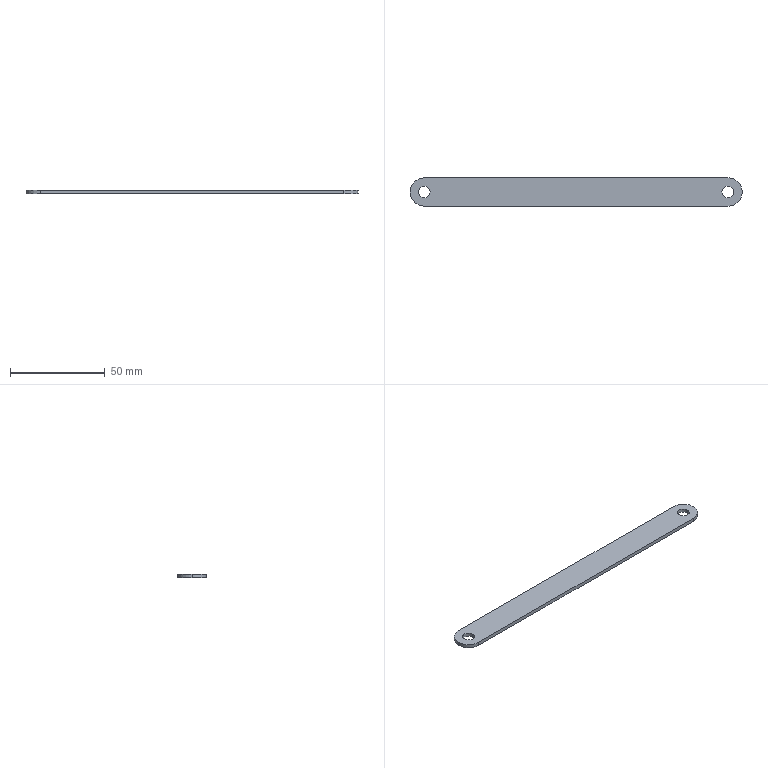Part | SolidWorks | features FlatPattern 1, SMBaseFlange 1, SheetMetal 1 | 1 solid | 11 faces | box 175 x 15 x 2 mm | volume 5033 mm3 | cylinder 7 | plane 4 | commonest cylinder face diameters 6.2 x4 15 x3
STEP:
#1=CARTESIAN_POINT('',(-3.1,7.5,2.));
#2=VERTEX_POINT('',#1);
#3=CARTESIAN_POINT('',(3.1,7.5,2.));
#4=VERTEX_POINT('',#3);
#5=CARTESIAN_POINT('',(0.,7.5,2.));
#6=DIRECTION('',(0.,0.,1.));
#7=DIRECTION('',(1.,0.,0.));
#8=AXIS2_PLACEMENT_3D('',#5,#6,#7);
#9=CIRCLE('',#8,3.1);
#10=EDGE_CURVE('',#2,#4,#9,.T.);
#11=ORIENTED_EDGE('',*,*,#10,.T.);
#12=CARTESIAN_POINT('',(3.1,7.5,0.));
#13=VERTEX_POINT('',#12);
#14=CARTESIAN_POINT('',(3.1,7.5,2.));
#15=DIRECTION('',(0.,0.,-1.));
#16=VECTOR('',#15,1000.);
#17=LINE('',#14,#16);
#18=EDGE_CURVE('',#4,#13,#17,.T.);
#19=ORIENTED_EDGE('',*,*,#18,.T.);
#20=CARTESIAN_POINT('',(-3.1,7.5,0.));
#21=VERTEX_POINT('',#20);
#22=CARTESIAN_POINT('',(0.,7.5,0.));
#23=DIRECTION('',(0.,0.,1.));
#24=DIRECTION('',(1.,0.,0.));
#25=AXIS2_PLACEMENT_3D('',#22,#23,#24);
#26=CIRCLE('',#25,3.1);
#27=EDGE_CURVE('',#21,#13,#26,.T.);
#28=ORIENTED_EDGE('',*,*,#27,.F.);
#29=CARTESIAN_POINT('',(-3.1,7.5,2.));
#30=DIRECTION('',(0.,0.,-1.));
#31=VECTOR('',#30,1000.);
#32=LINE('',#29,#31);
#33=EDGE_CURVE('',#2,#21,#32,.T.);
#34=ORIENTED_EDGE('',*,*,#33,.F.);
#35=EDGE_LOOP('',(#11,#19,#28,#34));
#36=FACE_OUTER_BOUND('',#35,.T.);
#37=CARTESIAN_POINT('',(0.,7.5,2.));
#38=DIRECTION('',(0.,0.,-1.));
#39=DIRECTION('',(-1.,0.,0.));
#40=AXIS2_PLACEMENT_3D('',#37,#38,#39);
#41=CYLINDRICAL_SURFACE('',#40,3.1);
#42=ADVANCED_FACE('',(#36),#41,.F.);
#43=CARTESIAN_POINT('',(-163.1,7.5,2.));
#44=VERTEX_POINT('',#43);
#45=CARTESIAN_POINT('',(-156.9,7.5,2.));
#46=VERTEX_POINT('',#45);
#47=CARTESIAN_POINT('',(-160.,7.5,2.));
#48=DIRECTION('',(0.,0.,1.));
#49=DIRECTION('',(1.,0.,0.));
#50=AXIS2_PLACEMENT_3D('',#47,#48,#49);
#51=CIRCLE('',#50,3.1);
#52=EDGE_CURVE('',#44,#46,#51,.T.);
#53=ORIENTED_EDGE('',*,*,#52,.T.);
#54=CARTESIAN_POINT('',(-156.9,7.5,0.));
#55=VERTEX_POINT('',#54);
#56=CARTESIAN_POINT('',(-156.9,7.5,2.));
#57=DIRECTION('',(0.,0.,-1.));
#58=VECTOR('',#57,1000.);
#59=LINE('',#56,#58);
#60=EDGE_CURVE('',#46,#55,#59,.T.);
#61=ORIENTED_EDGE('',*,*,#60,.T.);
#62=CARTESIAN_POINT('',(-163.1,7.5,0.));
#63=VERTEX_POINT('',#62);
#64=CARTESIAN_POINT('',(-160.,7.5,0.));
#65=DIRECTION('',(0.,0.,1.));
#66=DIRECTION('',(1.,0.,0.));
#67=AXIS2_PLACEMENT_3D('',#64,#65,#66);
#68=CIRCLE('',#67,3.1);
#69=EDGE_CURVE('',#63,#55,#68,.T.);
#70=ORIENTED_EDGE('',*,*,#69,.F.);
#71=CARTESIAN_POINT('',(-163.1,7.5,2.));
#72=DIRECTION('',(0.,0.,-1.));
#73=VECTOR('',#72,1000.);
#74=LINE('',#71,#73);
#75=EDGE_CURVE('',#44,#63,#74,.T.);
#76=ORIENTED_EDGE('',*,*,#75,.F.);
#77=EDGE_LOOP('',(#53,#61,#70,#76));
#78=FACE_OUTER_BOUND('',#77,.T.);
#79=CARTESIAN_POINT('',(-160.,7.5,2.));
#80=DIRECTION('',(0.,0.,-1.));
#81=DIRECTION('',(-1.,0.,0.));
#82=AXIS2_PLACEMENT_3D('',#79,#80,#81);
#83=CYLINDRICAL_SURFACE('',#82,3.1);
#84=ADVANCED_FACE('',(#78),#83,.F.);
#85=CARTESIAN_POINT('',(-167.5,7.5,2.));
#86=VERTEX_POINT('',#85);
#87=CARTESIAN_POINT('',(-160.,0.,2.));
#88=VERTEX_POINT('',#87);
#89=CARTESIAN_POINT('',(-160.,7.5,2.));
#90=DIRECTION('',(0.,0.,1.));
#91=DIRECTION('',(1.,0.,0.));
#92=AXIS2_PLACEMENT_3D('',#89,#90,#91);
#93=CIRCLE('',#92,7.5);
#94=EDGE_CURVE('',#86,#88,#93,.T.);
#95=ORIENTED_EDGE('',*,*,#94,.F.);
#96=CARTESIAN_POINT('',(-167.5,7.5,0.));
#97=VERTEX_POINT('',#96);
#98=CARTESIAN_POINT('',(-167.5,7.5,2.));
#99=DIRECTION('',(0.,0.,-1.));
#100=VECTOR('',#99,1000.);
#101=LINE('',#98,#100);
#102=EDGE_CURVE('',#86,#97,#101,.T.);
#103=ORIENTED_EDGE('',*,*,#102,.T.);
#104=CARTESIAN_POINT('',(-160.,0.,0.));
#105=VERTEX_POINT('',#104);
#106=CARTESIAN_POINT('',(-160.,7.5,0.));
#107=DIRECTION('',(0.,0.,1.));
#108=DIRECTION('',(1.,0.,0.));
#109=AXIS2_PLACEMENT_3D('',#106,#107,#108);
#110=CIRCLE('',#109,7.5);
#111=EDGE_CURVE('',#97,#105,#110,.T.);
#112=ORIENTED_EDGE('',*,*,#111,.T.);
#113=CARTESIAN_POINT('',(-160.,0.,2.));
#114=DIRECTION('',(0.,0.,-1.));
#115=VECTOR('',#114,1000.);
#116=LINE('',#113,#115);
#117=EDGE_CURVE('',#88,#105,#116,.T.);
#118=ORIENTED_EDGE('',*,*,#117,.F.);
#119=EDGE_LOOP('',(#95,#103,#112,#118));
#120=FACE_OUTER_BOUND('',#119,.T.);
#121=CARTESIAN_POINT('',(-160.,7.5,2.));
#122=DIRECTION('',(0.,0.,-1.));
#123=DIRECTION('',(-1.,0.,0.));
#124=AXIS2_PLACEMENT_3D('',#121,#122,#123);
#125=CYLINDRICAL_SURFACE('',#124,7.5);
#126=ADVANCED_FACE('',(#120),#125,.T.);
#127=ORIENTED_EDGE('',*,*,#52,.F.);
#128=CARTESIAN_POINT('',(-160.,7.5,2.));
#129=DIRECTION('',(0.,0.,1.));
#130=DIRECTION('',(1.,0.,0.));
#131=AXIS2_PLACEMENT_3D('',#128,#129,#130);
#132=CIRCLE('',#131,3.1);
#133=EDGE_CURVE('',#46,#44,#132,.T.);
#134=ORIENTED_EDGE('',*,*,#133,.F.);
#135=EDGE_LOOP('',(#127,#134));
#136=FACE_BOUND('',#135,.T.);
#137=CARTESIAN_POINT('',(0.,0.,2.));
#138=VERTEX_POINT('',#137);
#139=CARTESIAN_POINT('',(0.,15.,2.));
#140=VERTEX_POINT('',#139);
#141=CARTESIAN_POINT('',(0.,7.5,2.));
#142=DIRECTION('',(0.,0.,1.));
#143=DIRECTION('',(-1.,0.,0.));
#144=AXIS2_PLACEMENT_3D('',#141,#142,#143);
#145=CIRCLE('',#144,7.5);
#146=EDGE_CURVE('',#138,#140,#145,.T.);
#147=ORIENTED_EDGE('',*,*,#146,.T.);
#148=CARTESIAN_POINT('',(-160.,15.,2.));
#149=VERTEX_POINT('',#148);
#150=CARTESIAN_POINT('',(0.,15.,2.));
#151=DIRECTION('',(-1.,0.,0.));
#152=VECTOR('',#151,1000.);
#153=LINE('',#150,#152);
#154=EDGE_CURVE('',#140,#149,#153,.T.);
#155=ORIENTED_EDGE('',*,*,#154,.T.);
#156=CARTESIAN_POINT('',(-160.,7.5,2.));
#157=DIRECTION('',(0.,0.,1.));
#158=DIRECTION('',(1.,0.,0.));
#159=AXIS2_PLACEMENT_3D('',#156,#157,#158);
#160=CIRCLE('',#159,7.5);
#161=EDGE_CURVE('',#149,#86,#160,.T.);
#162=ORIENTED_EDGE('',*,*,#161,.T.);
#163=ORIENTED_EDGE('',*,*,#94,.T.);
#164=CARTESIAN_POINT('',(0.,0.,2.));
#165=DIRECTION('',(1.,0.,0.));
#166=VECTOR('',#165,1000.);
#167=LINE('',#164,#166);
#168=EDGE_CURVE('',#88,#138,#167,.T.);
#169=ORIENTED_EDGE('',*,*,#168,.T.);
#170=EDGE_LOOP('',(#147,#155,#162,#163,#169));
#171=FACE_OUTER_BOUND('',#170,.T.);
#172=ORIENTED_EDGE('',*,*,#10,.F.);
#173=CARTESIAN_POINT('',(0.,7.5,2.));
#174=DIRECTION('',(0.,0.,1.));
#175=DIRECTION('',(1.,0.,0.));
#176=AXIS2_PLACEMENT_3D('',#173,#174,#175);
#177=CIRCLE('',#176,3.1);
#178=EDGE_CURVE('',#4,#2,#177,.T.);
#179=ORIENTED_EDGE('',*,*,#178,.F.);
#180=EDGE_LOOP('',(#172,#179));
#181=FACE_BOUND('',#180,.T.);
#182=CARTESIAN_POINT('',(0.,7.5,2.));
#183=DIRECTION('',(0.,0.,-1.));
#184=DIRECTION('',(-1.,0.,0.));
#185=AXIS2_PLACEMENT_3D('',#182,#183,#184);
#186=PLANE('',#185);
#187=ADVANCED_FACE('',(#136,#171,#181),#186,.F.);
#188=ORIENTED_EDGE('',*,*,#69,.T.);
#189=CARTESIAN_POINT('',(-160.,7.5,0.));
#190=DIRECTION('',(0.,0.,1.));
#191=DIRECTION('',(1.,0.,0.));
#192=AXIS2_PLACEMENT_3D('',#189,#190,#191);
#193=CIRCLE('',#192,3.1);
#194=EDGE_CURVE('',#55,#63,#193,.T.);
#195=ORIENTED_EDGE('',*,*,#194,.T.);
#196=EDGE_LOOP('',(#188,#195));
#197=FACE_BOUND('',#196,.T.);
#198=CARTESIAN_POINT('',(0.,0.,0.));
#199=VERTEX_POINT('',#198);
#200=CARTESIAN_POINT('',(0.,15.,0.));
#201=VERTEX_POINT('',#200);
#202=CARTESIAN_POINT('',(0.,7.5,0.));
#203=DIRECTION('',(0.,0.,1.));
#204=DIRECTION('',(-1.,0.,0.));
#205=AXIS2_PLACEMENT_3D('',#202,#203,#204);
#206=CIRCLE('',#205,7.5);
#207=EDGE_CURVE('',#199,#201,#206,.T.);
#208=ORIENTED_EDGE('',*,*,#207,.F.);
#209=CARTESIAN_POINT('',(0.,0.,0.));
#210=DIRECTION('',(1.,0.,0.));
#211=VECTOR('',#210,1000.);
#212=LINE('',#209,#211);
#213=EDGE_CURVE('',#105,#199,#212,.T.);
#214=ORIENTED_EDGE('',*,*,#213,.F.);
#215=ORIENTED_EDGE('',*,*,#111,.F.);
#216=CARTESIAN_POINT('',(-160.,15.,0.));
#217=VERTEX_POINT('',#216);
#218=CARTESIAN_POINT('',(-160.,7.5,0.));
#219=DIRECTION('',(0.,0.,1.));
#220=DIRECTION('',(1.,0.,0.));
#221=AXIS2_PLACEMENT_3D('',#218,#219,#220);
#222=CIRCLE('',#221,7.5);
#223=EDGE_CURVE('',#217,#97,#222,.T.);
#224=ORIENTED_EDGE('',*,*,#223,.F.);
#225=CARTESIAN_POINT('',(0.,15.,0.));
#226=DIRECTION('',(-1.,0.,0.));
#227=VECTOR('',#226,1000.);
#228=LINE('',#225,#227);
#229=EDGE_CURVE('',#201,#217,#228,.T.);
#230=ORIENTED_EDGE('',*,*,#229,.F.);
#231=EDGE_LOOP('',(#208,#214,#215,#224,#230));
#232=FACE_OUTER_BOUND('',#231,.T.);
#233=ORIENTED_EDGE('',*,*,#27,.T.);
#234=CARTESIAN_POINT('',(0.,7.5,0.));
#235=DIRECTION('',(0.,0.,1.));
#236=DIRECTION('',(1.,0.,0.));
#237=AXIS2_PLACEMENT_3D('',#234,#235,#236);
#238=CIRCLE('',#237,3.1);
#239=EDGE_CURVE('',#13,#21,#238,.T.);
#240=ORIENTED_EDGE('',*,*,#239,.T.);
#241=EDGE_LOOP('',(#233,#240));
#242=FACE_BOUND('',#241,.T.);
#243=CARTESIAN_POINT('',(0.,7.5,0.));
#244=DIRECTION('',(0.,0.,-1.));
#245=DIRECTION('',(-1.,0.,0.));
#246=AXIS2_PLACEMENT_3D('',#243,#244,#245);
#247=PLANE('',#246);
#248=ADVANCED_FACE('',(#197,#232,#242),#247,.T.);
#249=ORIENTED_EDGE('',*,*,#207,.T.);
#250=CARTESIAN_POINT('',(0.,15.,2.));
#251=DIRECTION('',(0.,0.,-1.));
#252=VECTOR('',#251,1000.);
#253=LINE('',#250,#252);
#254=EDGE_CURVE('',#140,#201,#253,.T.);
#255=ORIENTED_EDGE('',*,*,#254,.F.);
#256=ORIENTED_EDGE('',*,*,#146,.F.);
#257=CARTESIAN_POINT('',(0.,0.,2.));
#258=DIRECTION('',(0.,0.,-1.));
#259=VECTOR('',#258,1000.);
#260=LINE('',#257,#259);
#261=EDGE_CURVE('',#138,#199,#260,.T.);
#262=ORIENTED_EDGE('',*,*,#261,.T.);
#263=EDGE_LOOP('',(#249,#255,#256,#262));
#264=FACE_OUTER_BOUND('',#263,.T.);
#265=CARTESIAN_POINT('',(0.,7.5,2.));
#266=DIRECTION('',(0.,0.,-1.));
#267=DIRECTION('',(-1.,0.,0.));
#268=AXIS2_PLACEMENT_3D('',#265,#266,#267);
#269=CYLINDRICAL_SURFACE('',#268,7.5);
#270=ADVANCED_FACE('',(#264),#269,.T.);
#271=ORIENTED_EDGE('',*,*,#229,.T.);
#272=CARTESIAN_POINT('',(-160.,15.,2.));
#273=DIRECTION('',(0.,0.,-1.));
#274=VECTOR('',#273,1000.);
#275=LINE('',#272,#274);
#276=EDGE_CURVE('',#149,#217,#275,.T.);
#277=ORIENTED_EDGE('',*,*,#276,.F.);
#278=ORIENTED_EDGE('',*,*,#154,.F.);
#279=ORIENTED_EDGE('',*,*,#254,.T.);
#280=EDGE_LOOP('',(#271,#277,#278,#279));
#281=FACE_OUTER_BOUND('',#280,.T.);
#282=CARTESIAN_POINT('',(0.,15.,2.));
#283=DIRECTION('',(0.,-1.,0.));
#284=DIRECTION('',(1.,0.,0.));
#285=AXIS2_PLACEMENT_3D('',#282,#283,#284);
#286=PLANE('',#285);
#287=ADVANCED_FACE('',(#281),#286,.F.);
#288=ORIENTED_EDGE('',*,*,#102,.F.);
#289=ORIENTED_EDGE('',*,*,#161,.F.);
#290=ORIENTED_EDGE('',*,*,#276,.T.);
#291=ORIENTED_EDGE('',*,*,#223,.T.);
#292=EDGE_LOOP('',(#288,#289,#290,#291));
#293=FACE_OUTER_BOUND('',#292,.T.);
#294=CARTESIAN_POINT('',(-160.,7.5,2.));
#295=DIRECTION('',(0.,0.,-1.));
#296=DIRECTION('',(-1.,0.,0.));
#297=AXIS2_PLACEMENT_3D('',#294,#295,#296);
#298=CYLINDRICAL_SURFACE('',#297,7.5);
#299=ADVANCED_FACE('',(#293),#298,.T.);
#300=ORIENTED_EDGE('',*,*,#213,.T.);
#301=ORIENTED_EDGE('',*,*,#261,.F.);
#302=ORIENTED_EDGE('',*,*,#168,.F.);
#303=ORIENTED_EDGE('',*,*,#117,.T.);
#304=EDGE_LOOP('',(#300,#301,#302,#303));
#305=FACE_OUTER_BOUND('',#304,.T.);
#306=CARTESIAN_POINT('',(0.,0.,2.));
#307=DIRECTION('',(0.,1.,0.));
#308=DIRECTION('',(-1.,0.,0.));
#309=AXIS2_PLACEMENT_3D('',#306,#307,#308);
#310=PLANE('',#309);
#311=ADVANCED_FACE('',(#305),#310,.F.);
#312=ORIENTED_EDGE('',*,*,#60,.F.);
#313=ORIENTED_EDGE('',*,*,#133,.T.);
#314=ORIENTED_EDGE('',*,*,#75,.T.);
#315=ORIENTED_EDGE('',*,*,#194,.F.);
#316=EDGE_LOOP('',(#312,#313,#314,#315));
#317=FACE_OUTER_BOUND('',#316,.T.);
#318=CARTESIAN_POINT('',(-160.,7.5,2.));
#319=DIRECTION('',(0.,0.,-1.));
#320=DIRECTION('',(-1.,0.,0.));
#321=AXIS2_PLACEMENT_3D('',#318,#319,#320);
#322=CYLINDRICAL_SURFACE('',#321,3.1);
#323=ADVANCED_FACE('',(#317),#322,.F.);
#324=ORIENTED_EDGE('',*,*,#18,.F.);
#325=ORIENTED_EDGE('',*,*,#178,.T.);
#326=ORIENTED_EDGE('',*,*,#33,.T.);
#327=ORIENTED_EDGE('',*,*,#239,.F.);
#328=EDGE_LOOP('',(#324,#325,#326,#327));
#329=FACE_OUTER_BOUND('',#328,.T.);
#330=CARTESIAN_POINT('',(0.,7.5,2.));
#331=DIRECTION('',(0.,0.,-1.));
#332=DIRECTION('',(-1.,0.,0.));
#333=AXIS2_PLACEMENT_3D('',#330,#331,#332);
#334=CYLINDRICAL_SURFACE('',#333,3.1);
#335=ADVANCED_FACE('',(#329),#334,.F.);
#336=CLOSED_SHELL('',(#42,#84,#126,#187,#248,#270,#287,#299,#311,#323,#335));
#337=MANIFOLD_SOLID_BREP('',#336);
#338=CARTESIAN_POINT('',(0.,0.,0.));
#339=DIRECTION('',(0.,0.,1.));
#340=DIRECTION('',(1.,0.,0.));
#341=AXIS2_PLACEMENT_3D('',#338,#339,#340);
#342=(LENGTH_UNIT()NAMED_UNIT(*)SI_UNIT(.MILLI.,.METRE.));
#343=UNCERTAINTY_MEASURE_WITH_UNIT(LENGTH_MEASURE(0.00001),#342,'','');
#344=(NAMED_UNIT(*)PLANE_ANGLE_UNIT()SI_UNIT($,.RADIAN.));
#345=(NAMED_UNIT(*)SI_UNIT($,.STERADIAN.)SOLID_ANGLE_UNIT());
#346=(GEOMETRIC_REPRESENTATION_CONTEXT(3)GLOBAL_UNCERTAINTY_ASSIGNED_CONTEXT((#343))GLOBAL_UNIT_ASSIGNED_CONTEXT((#342,#344,#345))REPRESENTATION_CONTEXT('',''));
#347=ADVANCED_BREP_SHAPE_REPRESENTATION('',(#337,#341),#346);